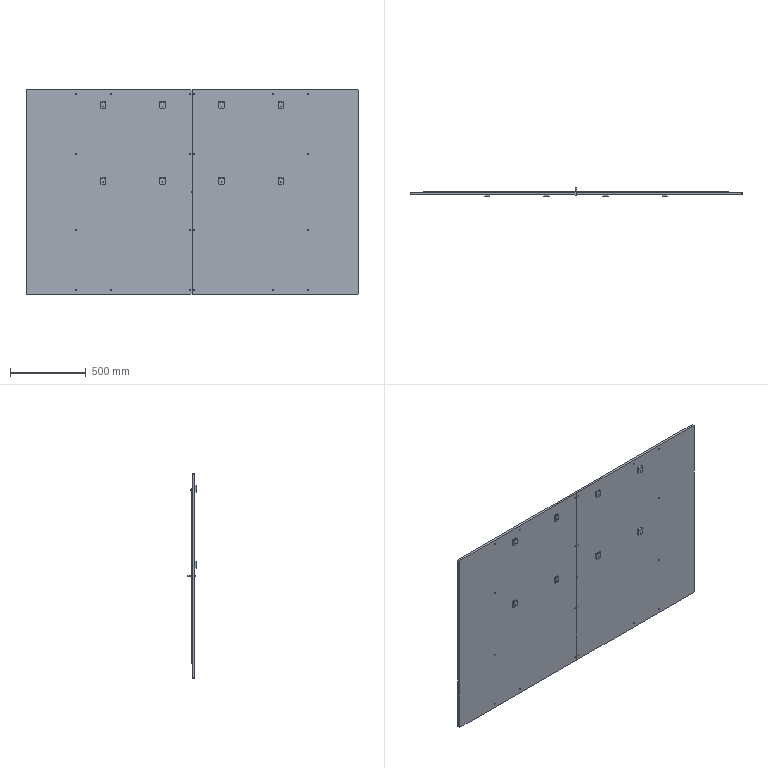Part | SolidWorks | features ReferencePattern 7, DerivedHolePattern 1 | 29 solids | 860 faces | box 2190 x 55.4 x 1350 mm | volume 56366306 mm3 | cylinder 406 | plane 358 | cone 64 | spline 32 | commonest cylinder face diameters 10 x54 4.2 x48 6.6 x40 11 x40 5.5 x32 6.1 x32